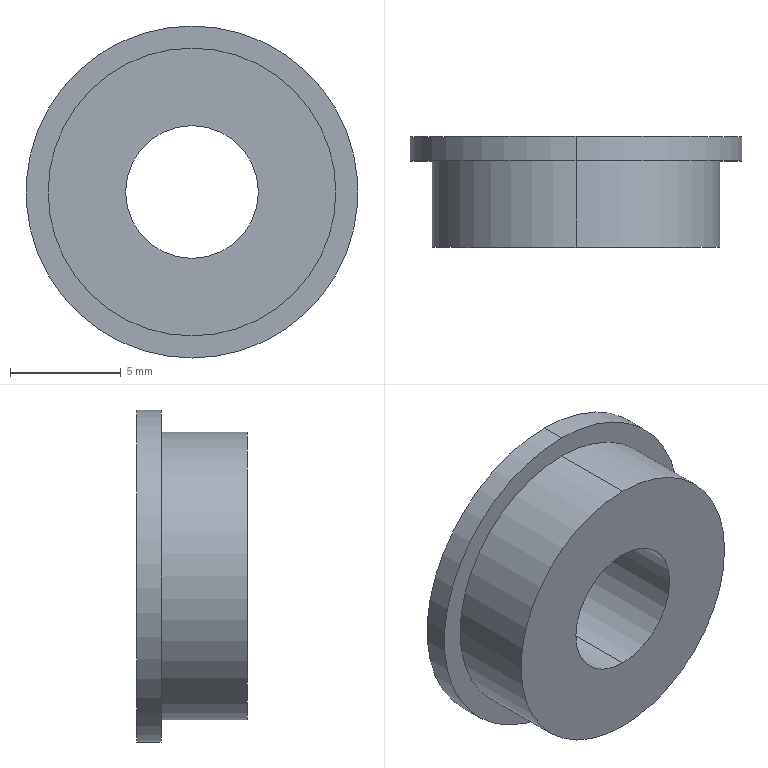Part | NX | features BREP 1 | 1 solid | 9 faces | box 15 x 5 x 15 mm | volume 570.67 mm3 | cylinder 6 | plane 3 | commonest cylinder face diameters 6 x2 13 x2 15 x2
STEP:
#1=CARTESIAN_POINT('',(0.,5.,-3.));
#2=VERTEX_POINT('',#1);
#3=CARTESIAN_POINT('',(0.,5.,3.));
#4=VERTEX_POINT('',#3);
#5=CARTESIAN_POINT('',(0.,5.,0.));
#6=DIRECTION('',(0.,-1.,0.));
#7=DIRECTION('',(0.,0.,-1.));
#8=AXIS2_PLACEMENT_3D('',#5,#6,#7);
#9=CIRCLE('',#8,3.);
#10=EDGE_CURVE('',#2,#4,#9,.T.);
#11=ORIENTED_EDGE('',*,*,#10,.T.);
#12=CARTESIAN_POINT('',(0.,5.,0.));
#13=DIRECTION('',(0.,-1.,0.));
#14=DIRECTION('',(0.,0.,-1.));
#15=AXIS2_PLACEMENT_3D('',#12,#13,#14);
#16=CIRCLE('',#15,3.);
#17=EDGE_CURVE('',#4,#2,#16,.T.);
#18=ORIENTED_EDGE('',*,*,#17,.T.);
#19=EDGE_LOOP('',(#11,#18));
#20=FACE_BOUND('',#19,.T.);
#21=CARTESIAN_POINT('',(0.,5.,-7.5));
#22=VERTEX_POINT('',#21);
#23=CARTESIAN_POINT('',(0.,5.,7.5));
#24=VERTEX_POINT('',#23);
#25=CARTESIAN_POINT('',(0.,5.,0.));
#26=DIRECTION('',(0.,-1.,0.));
#27=DIRECTION('',(0.,0.,-1.));
#28=AXIS2_PLACEMENT_3D('',#25,#26,#27);
#29=CIRCLE('',#28,7.5);
#30=EDGE_CURVE('',#22,#24,#29,.T.);
#31=ORIENTED_EDGE('',*,*,#30,.F.);
#32=CARTESIAN_POINT('',(0.,5.,0.));
#33=DIRECTION('',(0.,-1.,0.));
#34=DIRECTION('',(0.,0.,-1.));
#35=AXIS2_PLACEMENT_3D('',#32,#33,#34);
#36=CIRCLE('',#35,7.5);
#37=EDGE_CURVE('',#24,#22,#36,.T.);
#38=ORIENTED_EDGE('',*,*,#37,.F.);
#39=EDGE_LOOP('',(#31,#38));
#40=FACE_BOUND('',#39,.T.);
#41=CARTESIAN_POINT('',(-3.,5.,0.));
#42=DIRECTION('',(0.,-1.,0.));
#43=DIRECTION('',(0.,0.,-1.));
#44=AXIS2_PLACEMENT_3D('',#41,#42,#43);
#45=PLANE('',#44);
#46=ADVANCED_FACE('',(#20,#40),#45,.F.);
#47=CARTESIAN_POINT('',(0.,0.,3.));
#48=VERTEX_POINT('',#47);
#49=CARTESIAN_POINT('',(0.,0.,3.));
#50=DIRECTION('',(0.,-1.,0.));
#51=VECTOR('',#50,1000.);
#52=LINE('',#49,#51);
#53=EDGE_CURVE('',#4,#48,#52,.T.);
#54=ORIENTED_EDGE('',*,*,#53,.F.);
#55=ORIENTED_EDGE('',*,*,#10,.F.);
#56=CARTESIAN_POINT('',(0.,0.,-3.));
#57=VERTEX_POINT('',#56);
#58=CARTESIAN_POINT('',(0.,0.,-3.));
#59=DIRECTION('',(0.,-1.,0.));
#60=VECTOR('',#59,1000.);
#61=LINE('',#58,#60);
#62=EDGE_CURVE('',#2,#57,#61,.T.);
#63=ORIENTED_EDGE('',*,*,#62,.T.);
#64=CARTESIAN_POINT('',(0.,0.,0.));
#65=DIRECTION('',(0.,-1.,0.));
#66=DIRECTION('',(0.,0.,-1.));
#67=AXIS2_PLACEMENT_3D('',#64,#65,#66);
#68=CIRCLE('',#67,3.);
#69=EDGE_CURVE('',#57,#48,#68,.T.);
#70=ORIENTED_EDGE('',*,*,#69,.T.);
#71=EDGE_LOOP('',(#54,#55,#63,#70));
#72=FACE_BOUND('',#71,.T.);
#73=CARTESIAN_POINT('',(0.,0.,0.));
#74=DIRECTION('',(0.,-1.,0.));
#75=DIRECTION('',(0.,0.,-1.));
#76=AXIS2_PLACEMENT_3D('',#73,#74,#75);
#77=CYLINDRICAL_SURFACE('',#76,3.);
#78=ADVANCED_FACE('',(#72),#77,.F.);
#79=CARTESIAN_POINT('',(0.,0.,-6.5));
#80=VERTEX_POINT('',#79);
#81=CARTESIAN_POINT('',(0.,0.,6.5));
#82=VERTEX_POINT('',#81);
#83=CARTESIAN_POINT('',(0.,0.,0.));
#84=DIRECTION('',(0.,-1.,0.));
#85=DIRECTION('',(0.,0.,-1.));
#86=AXIS2_PLACEMENT_3D('',#83,#84,#85);
#87=CIRCLE('',#86,6.5);
#88=EDGE_CURVE('',#80,#82,#87,.T.);
#89=ORIENTED_EDGE('',*,*,#88,.T.);
#90=CARTESIAN_POINT('',(0.,0.,0.));
#91=DIRECTION('',(0.,-1.,0.));
#92=DIRECTION('',(0.,0.,-1.));
#93=AXIS2_PLACEMENT_3D('',#90,#91,#92);
#94=CIRCLE('',#93,6.5);
#95=EDGE_CURVE('',#82,#80,#94,.T.);
#96=ORIENTED_EDGE('',*,*,#95,.T.);
#97=EDGE_LOOP('',(#89,#96));
#98=FACE_BOUND('',#97,.T.);
#99=ORIENTED_EDGE('',*,*,#69,.F.);
#100=CARTESIAN_POINT('',(0.,0.,0.));
#101=DIRECTION('',(0.,-1.,0.));
#102=DIRECTION('',(0.,0.,-1.));
#103=AXIS2_PLACEMENT_3D('',#100,#101,#102);
#104=CIRCLE('',#103,3.);
#105=EDGE_CURVE('',#48,#57,#104,.T.);
#106=ORIENTED_EDGE('',*,*,#105,.F.);
#107=EDGE_LOOP('',(#99,#106));
#108=FACE_BOUND('',#107,.T.);
#109=CARTESIAN_POINT('',(-6.5,0.,0.));
#110=DIRECTION('',(0.,1.,0.));
#111=DIRECTION('',(0.,0.,1.));
#112=AXIS2_PLACEMENT_3D('',#109,#110,#111);
#113=PLANE('',#112);
#114=ADVANCED_FACE('',(#98,#108),#113,.F.);
#115=CARTESIAN_POINT('',(0.,3.9,6.5));
#116=VERTEX_POINT('',#115);
#117=CARTESIAN_POINT('',(0.,0.,6.5));
#118=DIRECTION('',(0.,-1.,0.));
#119=VECTOR('',#118,1000.);
#120=LINE('',#117,#119);
#121=EDGE_CURVE('',#116,#82,#120,.T.);
#122=ORIENTED_EDGE('',*,*,#121,.F.);
#123=CARTESIAN_POINT('',(0.,3.9,-6.5));
#124=VERTEX_POINT('',#123);
#125=CARTESIAN_POINT('',(0.,3.9,0.));
#126=DIRECTION('',(0.,-1.,0.));
#127=DIRECTION('',(0.,0.,-1.));
#128=AXIS2_PLACEMENT_3D('',#125,#126,#127);
#129=CIRCLE('',#128,6.5);
#130=EDGE_CURVE('',#116,#124,#129,.T.);
#131=ORIENTED_EDGE('',*,*,#130,.T.);
#132=CARTESIAN_POINT('',(0.,0.,-6.5));
#133=DIRECTION('',(0.,-1.,0.));
#134=VECTOR('',#133,1000.);
#135=LINE('',#132,#134);
#136=EDGE_CURVE('',#124,#80,#135,.T.);
#137=ORIENTED_EDGE('',*,*,#136,.T.);
#138=ORIENTED_EDGE('',*,*,#95,.F.);
#139=EDGE_LOOP('',(#122,#131,#137,#138));
#140=FACE_BOUND('',#139,.T.);
#141=CARTESIAN_POINT('',(0.,0.,0.));
#142=DIRECTION('',(0.,-1.,0.));
#143=DIRECTION('',(0.,0.,-1.));
#144=AXIS2_PLACEMENT_3D('',#141,#142,#143);
#145=CYLINDRICAL_SURFACE('',#144,6.5);
#146=ADVANCED_FACE('',(#140),#145,.T.);
#147=CARTESIAN_POINT('',(0.,3.9,-7.5));
#148=VERTEX_POINT('',#147);
#149=CARTESIAN_POINT('',(0.,3.9,7.5));
#150=VERTEX_POINT('',#149);
#151=CARTESIAN_POINT('',(0.,3.9,0.));
#152=DIRECTION('',(0.,-1.,0.));
#153=DIRECTION('',(0.,0.,-1.));
#154=AXIS2_PLACEMENT_3D('',#151,#152,#153);
#155=CIRCLE('',#154,7.5);
#156=EDGE_CURVE('',#148,#150,#155,.T.);
#157=ORIENTED_EDGE('',*,*,#156,.T.);
#158=CARTESIAN_POINT('',(0.,3.9,0.));
#159=DIRECTION('',(0.,-1.,0.));
#160=DIRECTION('',(0.,0.,-1.));
#161=AXIS2_PLACEMENT_3D('',#158,#159,#160);
#162=CIRCLE('',#161,7.5);
#163=EDGE_CURVE('',#150,#148,#162,.T.);
#164=ORIENTED_EDGE('',*,*,#163,.T.);
#165=EDGE_LOOP('',(#157,#164));
#166=FACE_BOUND('',#165,.T.);
#167=CARTESIAN_POINT('',(0.,3.9,0.));
#168=DIRECTION('',(0.,-1.,0.));
#169=DIRECTION('',(0.,0.,-1.));
#170=AXIS2_PLACEMENT_3D('',#167,#168,#169);
#171=CIRCLE('',#170,6.5);
#172=EDGE_CURVE('',#124,#116,#171,.T.);
#173=ORIENTED_EDGE('',*,*,#172,.F.);
#174=ORIENTED_EDGE('',*,*,#130,.F.);
#175=EDGE_LOOP('',(#173,#174));
#176=FACE_BOUND('',#175,.T.);
#177=CARTESIAN_POINT('',(-7.5,3.9,0.));
#178=DIRECTION('',(0.,1.,0.));
#179=DIRECTION('',(0.,0.,1.));
#180=AXIS2_PLACEMENT_3D('',#177,#178,#179);
#181=PLANE('',#180);
#182=ADVANCED_FACE('',(#166,#176),#181,.F.);
#183=CARTESIAN_POINT('',(0.,0.,7.5));
#184=DIRECTION('',(0.,-1.,0.));
#185=VECTOR('',#184,1000.);
#186=LINE('',#183,#185);
#187=EDGE_CURVE('',#24,#150,#186,.T.);
#188=ORIENTED_EDGE('',*,*,#187,.F.);
#189=ORIENTED_EDGE('',*,*,#37,.T.);
#190=CARTESIAN_POINT('',(0.,0.,-7.5));
#191=DIRECTION('',(0.,-1.,0.));
#192=VECTOR('',#191,1000.);
#193=LINE('',#190,#192);
#194=EDGE_CURVE('',#22,#148,#193,.T.);
#195=ORIENTED_EDGE('',*,*,#194,.T.);
#196=ORIENTED_EDGE('',*,*,#163,.F.);
#197=EDGE_LOOP('',(#188,#189,#195,#196));
#198=FACE_BOUND('',#197,.T.);
#199=CARTESIAN_POINT('',(0.,0.,0.));
#200=DIRECTION('',(0.,-1.,0.));
#201=DIRECTION('',(0.,0.,-1.));
#202=AXIS2_PLACEMENT_3D('',#199,#200,#201);
#203=CYLINDRICAL_SURFACE('',#202,7.5);
#204=ADVANCED_FACE('',(#198),#203,.T.);
#205=ORIENTED_EDGE('',*,*,#30,.T.);
#206=ORIENTED_EDGE('',*,*,#187,.T.);
#207=ORIENTED_EDGE('',*,*,#156,.F.);
#208=ORIENTED_EDGE('',*,*,#194,.F.);
#209=EDGE_LOOP('',(#205,#206,#207,#208));
#210=FACE_BOUND('',#209,.T.);
#211=CARTESIAN_POINT('',(0.,0.,0.));
#212=DIRECTION('',(0.,-1.,0.));
#213=DIRECTION('',(0.,0.,-1.));
#214=AXIS2_PLACEMENT_3D('',#211,#212,#213);
#215=CYLINDRICAL_SURFACE('',#214,7.5);
#216=ADVANCED_FACE('',(#210),#215,.T.);
#217=ORIENTED_EDGE('',*,*,#172,.T.);
#218=ORIENTED_EDGE('',*,*,#121,.T.);
#219=ORIENTED_EDGE('',*,*,#88,.F.);
#220=ORIENTED_EDGE('',*,*,#136,.F.);
#221=EDGE_LOOP('',(#217,#218,#219,#220));
#222=FACE_BOUND('',#221,.T.);
#223=CARTESIAN_POINT('',(0.,0.,0.));
#224=DIRECTION('',(0.,-1.,0.));
#225=DIRECTION('',(0.,0.,-1.));
#226=AXIS2_PLACEMENT_3D('',#223,#224,#225);
#227=CYLINDRICAL_SURFACE('',#226,6.5);
#228=ADVANCED_FACE('',(#222),#227,.T.);
#229=ORIENTED_EDGE('',*,*,#17,.F.);
#230=ORIENTED_EDGE('',*,*,#53,.T.);
#231=ORIENTED_EDGE('',*,*,#105,.T.);
#232=ORIENTED_EDGE('',*,*,#62,.F.);
#233=EDGE_LOOP('',(#229,#230,#231,#232));
#234=FACE_BOUND('',#233,.T.);
#235=CARTESIAN_POINT('',(0.,0.,0.));
#236=DIRECTION('',(0.,-1.,0.));
#237=DIRECTION('',(0.,0.,-1.));
#238=AXIS2_PLACEMENT_3D('',#235,#236,#237);
#239=CYLINDRICAL_SURFACE('',#238,3.);
#240=ADVANCED_FACE('',(#234),#239,.F.);
#241=CLOSED_SHELL('',(#46,#78,#114,#146,#182,#204,#216,#228,#240));
#242=MANIFOLD_SOLID_BREP('',#241);
#243=(LENGTH_UNIT()NAMED_UNIT(*)SI_UNIT(.MILLI.,.METRE.));
#244=UNCERTAINTY_MEASURE_WITH_UNIT(LENGTH_MEASURE(0.00001),#243,'','');
#245=(NAMED_UNIT(*)PLANE_ANGLE_UNIT()SI_UNIT($,.RADIAN.));
#246=(NAMED_UNIT(*)SI_UNIT($,.STERADIAN.)SOLID_ANGLE_UNIT());
#247=(GEOMETRIC_REPRESENTATION_CONTEXT(3)GLOBAL_UNCERTAINTY_ASSIGNED_CONTEXT((#244))GLOBAL_UNIT_ASSIGNED_CONTEXT((#243,#245,#246))REPRESENTATION_CONTEXT('',''));
#248=ADVANCED_BREP_SHAPE_REPRESENTATION('',(#242),#247);